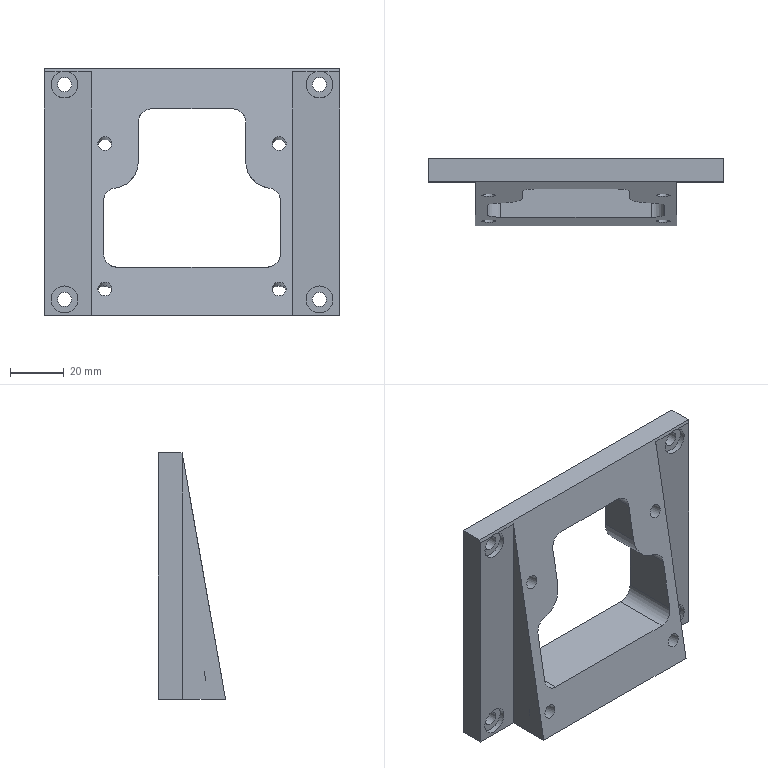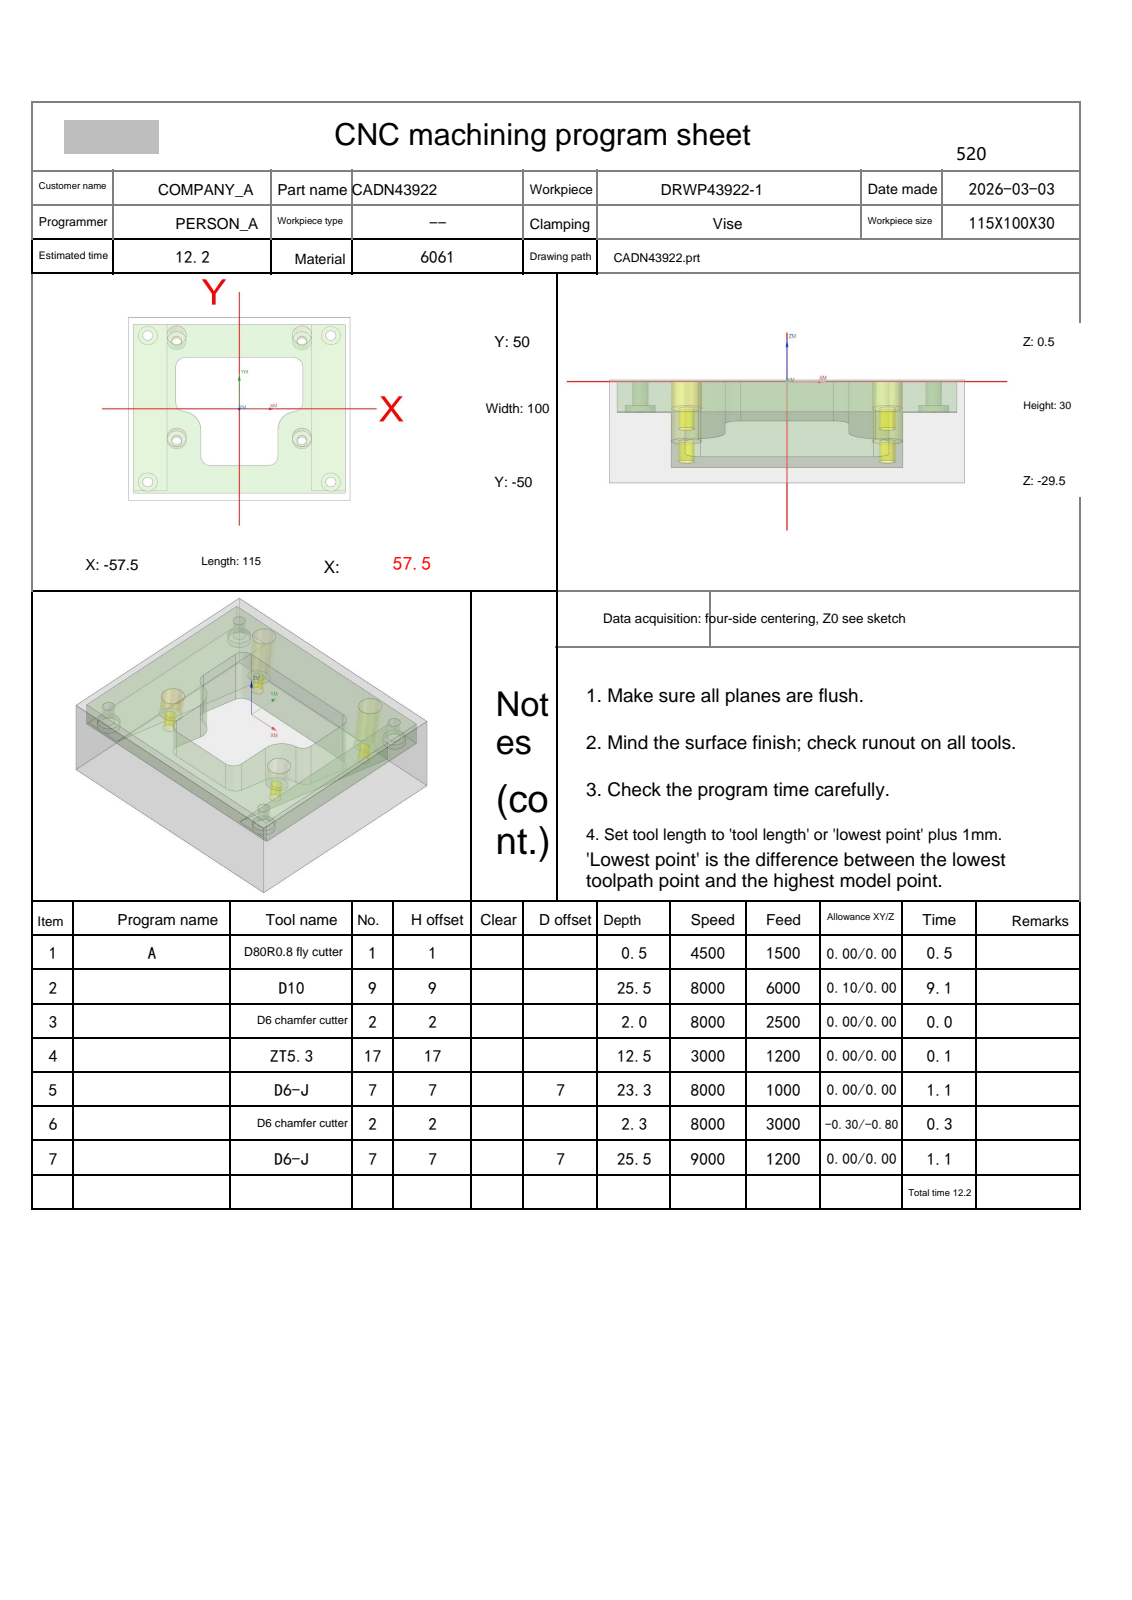NC program | NX | posted by the shop | part box 110 x 25 x 92 mm
Lines 36 to 1047 of 4607:
N2 T09 M06
(D10  D=10. R=0. H=09 ce=0.10 di=0.00)
G00 G90 G54 X0.0 Y-51.1 M03 S8000
G43 H09 Z50.
M08
Z.5
G01 X-55. Z.399 F6000.
G02 X-60.1 Y-46. Z.385 I0.0 J5.1
G01 Y46. Z.217
G02 X-55. Y51.1 Z.202 I5.1 J0.0
G01 X55. Z.001
G02 X60.1 Y46. Z-.014 I0.0 J-5.1
G01 Y-46. Z-.182
G02 X55. Y-51.1 Z-.196 I-5.1 J0.0
G01 X-55. Z-.397
G02 X-60.1 Y-46. Z-.412 I0.0 J5.1
G01 Y46. Z-.58
G02 X-55. Y51.1 Z-.595 I5.1 J0.0
G01 X55. Z-.796
G02 X60.1 Y46. Z-.81 I0.0 J-5.1
G01 Y-46. Z-.979
G02 X55. Y-51.1 Z-.993 I-5.1 J0.0
G01 X-55. Z-1.194
G02 X-60.1 Y-46. Z-1.209 I0.0 J5.1
G01 Y46. Z-1.377
G02 X-55. Y51.1 Z-1.392 I5.1 J0.0
G01 X55. Z-1.593
G02 X60.1 Y46. Z-1.607 I0.0 J-5.1
G01 Y-46. Z-1.775
G02 X55. Y-51.1 Z-1.79 I-5.1 J0.0
G01 X-55. Z-1.991
G02 X-60.1 Y-46. Z-2.006 I0.0 J5.1
G01 Y46. Z-2.174
G02 X-55. Y51.1 Z-2.189 I5.1 J0.0
G01 X55. Z-2.39
G02 X60.1 Y46. Z-2.404 I0.0 J-5.1
G01 Y-46. Z-2.572
G02 X55. Y-51.1 Z-2.587 I-5.1 J0.0
G01 X-55. Z-2.788
G02 X-60.1 Y-46. Z-2.803 I0.0 J5.1
G01 Y46. Z-2.971
G02 X-55. Y51.1 Z-2.985 I5.1 J0.0
G01 X55. Z-3.186
G02 X60.1 Y46. Z-3.201 I0.0 J-5.1
G01 Y-46. Z-3.369
G02 X55. Y-51.1 Z-3.384 I-5.1 J0.0
G01 X-55. Z-3.585
G02 X-60.1 Y-46. Z-3.6 I0.0 J5.1
G01 Y46. Z-3.768
G02 X-55. Y51.1 Z-3.782 I5.1 J0.0
G01 X55. Z-3.983
G02 X60.1 Y46. Z-3.998 I0.0 J-5.1
G01 Y-46. Z-4.166
G02 X55. Y-51.1 Z-4.181 I-5.1 J0.0
G01 X-55. Z-4.382
G02 X-60.1 Y-46. Z-4.396 I0.0 J5.1
G01 Y46. Z-4.565
G02 X-55. Y51.1 Z-4.579 I5.1 J0.0
G01 X55. Z-4.78
G02 X60.1 Y46. Z-4.795 I0.0 J-5.1
G01 Y-46. Z-4.963
G02 X55. Y-51.1 Z-4.978 I-5.1 J0.0
G01 X-55. Z-5.179
G02 X-60.1 Y-46. Z-5.193 I0.0 J5.1
G01 Y46. Z-5.361
G02 X-55. Y51.1 Z-5.376 I5.1 J0.0
G01 X55. Z-5.577
G02 X60.1 Y46. Z-5.592 I0.0 J-5.1
G01 Y-46. Z-5.76
G02 X55. Y-51.1 Z-5.774 I-5.1 J0.0
G01 X-55. Z-5.976
G02 X-60.1 Y-46. Z-5.99 I0.0 J5.1
G01 Y46. Z-6.158
G02 X-55. Y51.1 Z-6.173 I5.1 J0.0
G01 X55. Z-6.374
G02 X60.1 Y46. Z-6.389 I0.0 J-5.1
G01 Y-46. Z-6.557
G02 X55. Y-51.1 Z-6.571 I-5.1 J0.0
G01 X-55. Z-6.772
G02 X-60.1 Y-46. Z-6.787 I0.0 J5.1
G01 Y46. Z-6.955
G02 X-55. Y51.1 Z-6.97 I5.1 J0.0
G01 X55. Z-7.171
G02 X60.1 Y46. Z-7.185 I0.0 J-5.1
G01 Y-46. Z-7.354
G02 X55. Y-51.1 Z-7.368 I-5.1 J0.0
G01 X-55. Z-7.569
G02 X-60.1 Y-46. Z-7.584 I0.0 J5.1
G01 Y46. Z-7.752
G02 X-55. Y51.1 Z-7.767 I5.1 J0.0
G01 X55. Z-7.968
G02 X60.1 Y46. Z-7.982 I0.0 J-5.1
G01 Y-46. Z-8.15
G02 X55. Y-51.1 Z-8.165 I-5.1 J0.0
G01 X-55. Z-8.366
G02 X-60.1 Y-46. Z-8.381 I0.0 J5.1
G01 Y46. Z-8.549
G02 X-55. Y51.1 Z-8.564 I5.1 J0.0
G01 X55. Z-8.765
G02 X60.1 Y46. Z-8.779 I0.0 J-5.1
G01 Y-46. Z-8.947
G02 X55. Y-51.1 Z-8.962 I-5.1 J0.0
G01 X-55. Z-9.163
G02 X-60.1 Y-46. Z-9.178 I0.0 J5.1
G01 Y46. Z-9.346
G02 X-55. Y51.1 Z-9.36 I5.1 J0.0
G01 X55. Z-9.561
G02 X60.1 Y46. Z-9.576 I0.0 J-5.1
G01 Y-46. Z-9.744
G02 X55. Y-51.1 Z-9.759 I-5.1 J0.0
G01 X-55. Z-9.96
G02 X-60.1 Y-46. Z-9.975 I0.0 J5.1
G01 Y46. Z-10.143
G02 X-55. Y51.1 Z-10.157 I5.1 J0.0
G01 X55. Z-10.358
G02 X60.1 Y46. Z-10.373 I0.0 J-5.1
G01 Y-46. Z-10.541
G02 X55. Y-51.1 Z-10.556 I-5.1 J0.0
G01 X-55. Z-10.757
G02 X-60.1 Y-46. Z-10.771 I0.0 J5.1
G01 Y46. Z-10.94
G02 X-55. Y51.1 Z-10.954 I5.1 J0.0
G01 X55. Z-11.155
G02 X60.1 Y46. Z-11.17 I0.0 J-5.1
G01 Y-46. Z-11.338
G02 X55. Y-51.1 Z-11.353 I-5.1 J0.0
G01 X-55. Z-11.554
G02 X-60.1 Y-46. Z-11.568 I0.0 J5.1
G01 Y46. Z-11.736
G02 X-55. Y51.1 Z-11.751 I5.1 J0.0
G01 X55. Z-11.952
G02 X60.1 Y46. Z-11.967 I0.0 J-5.1
G01 Y-46. Z-12.135
G02 X55. Y-51.1 Z-12.149 I-5.1 J0.0
G01 X-55. Z-12.351
G02 X-60.1 Y-46. Z-12.365 I0.0 J5.1
G01 Y46. Z-12.533
G02 X-55. Y51.1 Z-12.548 I5.1 J0.0
G01 X55. Z-12.749
G02 X60.1 Y46. Z-12.764 I0.0 J-5.1
G01 Y-46. Z-12.932
G02 X55. Y-51.1 Z-12.946 I-5.1 J0.0
G01 X-55. Z-13.147
G02 X-60.1 Y-46. Z-13.162 I0.0 J5.1
G01 Y46. Z-13.33
G02 X-55. Y51.1 Z-13.345 I5.1 J0.0
G01 X55. Z-13.546
G02 X60.1 Y46. Z-13.56 I0.0 J-5.1
G01 Y-46. Z-13.729
G02 X55. Y-51.1 Z-13.743 I-5.1 J0.0
G01 X-55. Z-13.944
G02 X-60.1 Y-46. Z-13.959 I0.0 J5.1
G01 Y46. Z-14.127
G02 X-55. Y51.1 Z-14.142 I5.1 J0.0
G01 X55. Z-14.343
G02 X60.1 Y46. Z-14.357 I0.0 J-5.1
G01 Y-46. Z-14.525
G02 X55. Y-51.1 Z-14.54 I-5.1 J0.0
G01 X-55. Z-14.741
G02 X-60.1 Y-46. Z-14.756 I0.0 J5.1
G01 Y46. Z-14.924
G02 X-55. Y51.1 Z-14.939 I5.1 J0.0
G01 X55. Z-15.14
G02 X60.1 Y46. Z-15.154 I0.0 J-5.1
G01 Y-46. Z-15.322
G02 X55. Y-51.1 Z-15.337 I-5.1 J0.0
G01 X-55. Z-15.538
G02 X-60.1 Y-46. Z-15.553 I0.0 J5.1
G01 Y46. Z-15.721
G02 X-55. Y51.1 Z-15.735 I5.1 J0.0
G01 X55. Z-15.936
G02 X60.1 Y46. Z-15.951 I0.0 J-5.1
G01 Y-46. Z-16.119
G02 X55. Y-51.1 Z-16.134 I-5.1 J0.0
G01 X-55. Z-16.335
G02 X-60.1 Y-46. Z-16.35 I0.0 J5.1
G01 Y46. Z-16.518
G02 X-55. Y51.1 Z-16.532 I5.1 J0.0
G01 X55. Z-16.733
G02 X60.1 Y46. Z-16.748 I0.0 J-5.1
G01 Y-46. Z-16.916
G02 X55. Y-51.1 Z-16.931 I-5.1 J0.0
G01 X-55. Z-17.132
G02 X-60.1 Y-46. Z-17.146 I0.0 J5.1
G01 Y46. Z-17.315
G02 X-55. Y51.1 Z-17.329 I5.1 J0.0
G01 X55. Z-17.53
G02 X60.1 Y46. Z-17.545 I0.0 J-5.1
G01 Y-46. Z-17.713
G02 X55. Y-51.1 Z-17.728 I-5.1 J0.0
G01 X-55. Z-17.929
G02 X-60.1 Y-46. Z-17.943 I0.0 J5.1
G01 Y46. Z-18.111
G02 X-55. Y51.1 Z-18.126 I5.1 J0.0
G01 X55. Z-18.327
G02 X60.1 Y46. Z-18.342 I0.0 J-5.1
G01 Y-46. Z-18.51
G02 X55. Y-51.1 Z-18.524 I-5.1 J0.0
G01 X-55. Z-18.726
G02 X-60.1 Y-46. Z-18.74 I0.0 J5.1
G01 Y46. Z-18.908
G02 X-55. Y51.1 Z-18.923 I5.1 J0.0
G01 X55. Z-19.124
G02 X60.1 Y46. Z-19.139 I0.0 J-5.1
G01 Y-46. Z-19.307
G02 X55. Y-51.1 Z-19.321 I-5.1 J0.0
G01 X-55. Z-19.522
G02 X-60.1 Y-46. Z-19.537 I0.0 J5.1
G01 Y46. Z-19.705
G02 X-55. Y51.1 Z-19.72 I5.1 J0.0
G01 X55. Z-19.921
G02 X60.1 Y46. Z-19.935 I0.0 J-5.1
G01 Y-46. Z-20.104
G02 X55. Y-51.1 Z-20.118 I-5.1 J0.0
G01 X-55. Z-20.319
G02 X-60.1 Y-46. Z-20.334 I0.0 J5.1
G01 Y46. Z-20.502
G02 X-55. Y51.1 Z-20.517 I5.1 J0.0
G01 X55. Z-20.718
G02 X60.1 Y46. Z-20.732 I0.0 J-5.1
G01 Y-46. Z-20.9
G02 X55. Y-51.1 Z-20.915 I-5.1 J0.0
G01 X-55. Z-21.116
G02 X-60.1 Y-46. Z-21.131 I0.0 J5.1
G01 Y46. Z-21.299
G02 X-55. Y51.1 Z-21.314 I5.1 J0.0
G01 X55. Z-21.515
G02 X60.1 Y46. Z-21.529 I0.0 J-5.1
G01 Y-46. Z-21.697
G02 X55. Y-51.1 Z-21.712 I-5.1 J0.0
G01 X-55. Z-21.913
G02 X-60.1 Y-46. Z-21.928 I0.0 J5.1
G01 Y46. Z-22.096
G02 X-55. Y51.1 Z-22.11 I5.1 J0.0
G01 X55. Z-22.311
G02 X60.1 Y46. Z-22.326 I0.0 J-5.1
G01 Y-46. Z-22.494
G02 X55. Y-51.1 Z-22.509 I-5.1 J0.0
G01 X-55. Z-22.71
G02 X-60.1 Y-46. Z-22.725 I0.0 J5.1
G01 Y46. Z-22.893
G02 X-55. Y51.1 Z-22.907 I5.1 J0.0
G01 X55. Z-23.108
G02 X60.1 Y46. Z-23.123 I0.0 J-5.1
G01 Y-46. Z-23.291
G02 X55. Y-51.1 Z-23.306 I-5.1 J0.0
G01 X-55. Z-23.507
G02 X-60.1 Y-46. Z-23.521 I0.0 J5.1
G01 Y46. Z-23.69
G02 X-55. Y51.1 Z-23.704 I5.1 J0.0
G01 X55. Z-23.905
G02 X60.1 Y46. Z-23.92 I0.0 J-5.1
G01 Y-46. Z-24.088
G02 X55. Y-51.1 Z-24.103 I-5.1 J0.0
G01 X-55. Z-24.304
G02 X-60.1 Y-46. Z-24.318 I0.0 J5.1
G01 Y46. Z-24.486
G02 X-55. Y51.1 Z-24.501 I5.1 J0.0
G01 X55. Z-24.702
G02 X60.1 Y46. Z-24.717 I0.0 J-5.1
G01 Y-46. Z-24.885
G02 X55. Y-51.1 Z-24.899 I-5.1 J0.0
G01 X0.0 Z-25.
X-55.
G02 X-60.1 Y-46. I0.0 J5.1
G01 Y46.
G02 X-55. Y51.1 I5.1 J0.0
G01 X55.
G02 X60.1 Y46. I0.0 J-5.1
G01 Y-46.
G02 X55. Y-51.1 I-5.1 J0.0
G01 X0.0
X-.5
Z-24.
G00 Z50.
G00 G90 X-1.466 Y13.145 M03 S8000
Z10.5
Z1.5
G02 X-1.466 Y13.145 Z.018 I1.466 J4.255 F4000.
X-2.587 Y21.082 Z-.5 I1.466 J4.255
G01 X0.0 Y22.9
X27.9
Y3.587
G03 X14.9 Y-11.366 I2.1 J-14.953
G01 Y-25.9
X-14.9
Y-11.366
G03 X-27.9 Y3.587 I-15.1 J0.0
G01 Y22.9
X1.986
G02 X2.799 Y22.482 I0.0 J-1.
G01 X7.201 Y16.318
G03 X8.014 Y15.9 I.814 J.582
G01 X19.901
G02 X20.9 Y14.901 I-.001 J-1.
G01 Y13.66
G02 X20.631 Y12.978 I-1. J0.0
G01 X19.569 Y11.842
G03 X19.31 Y11.298 I.731 J-.683
G02 X17.61 Y9.268 I-2.476 J.347
G01 X10.909 Y7.08
G02 X10.133 Y6.957 I-.776 J2.377
X7.633 Y9.457 I0.0 J2.5
X9.357 Y11.833 I2.5 J0.0
G01 X16.058 Y14.021
G02 X16.834 Y14.145 I.776 J-2.377
X18.754 Y13.246 I0.0 J-2.5
G03 X18.916 Y13.091 I.768 J.64
G01 X20.507 Y11.876
G02 X20.9 Y11.082 I-.607 J-.795
G01 Y9.408
G02 X20.338 Y8.51 I-1. J.001
G03 X7.9 Y-11.366 I9.662 J-19.876
G01 Y-17.901
G02 X6.901 Y-18.9 I-1. J.001
G01 X-6.901
G02 X-7.9 Y-17.901 I.001 J1.
G01 Y-11.366
G03 X-20.338 Y8.51 I-22.1 J0.0
G02 X-20.9 Y9.408 I.438 J.899
G01 Y11.081
G02 X-20.507 Y11.876 I1. J0.0
G01 X-18.915 Y13.091
G03 X-18.754 Y13.245 I-.607 J.795
G02 X-16.834 Y14.145 I1.921 J-1.6
X-16.058 Y14.021 I0.0 J-2.5
G01 X-9.357 Y11.833
G02 X-7.633 Y9.457 I-.776 J-2.377
X-10.133 Y6.957 I-2.5 J0.0
X-10.909 Y7.08 I0.0 J2.5
G01 X-17.61 Y9.268
G02 X-19.31 Y11.298 I.776 J2.377
G03 X-19.569 Y11.842 I-.99 J-.139
G01 X-20.631 Y12.978
G02 X-20.9 Y13.66 I.731 J.682
G01 Y14.901
G02 X-19.901 Y15.9 I1. J-.001
G01 X1.975
G02 X2.798 Y15.468 I0.0 J-1.
G01 X7.38 Y8.827
G03 X7.538 Y8.648 I.823 J.568
G02 X7.874 Y7.9 I-.664 J-.748
X7.643 Y7.261 I-1. J0.0
G03 X.902 Y-11.012 I22.357 J-18.627
G02 X.002 Y-11.9 I-.9 J.012
G01 X-.004
G02 X-.902 Y-11.012 I.001 J.9
G03 X-7.643 Y7.261 I-29.098 J-.354
G02 X-7.874 Y7.9 I.769 J.639
X-6.875 Y8.9 I1. J0.0
G01 X5.
X5.5
G03 X12.5 Y15.9 I0.0 J7.
G01 Z.7
G00 Z3.
G01 X-1.466 Y13.145 F6000.
G00 Z1.
G02 X-1.466 Y13.145 Z-.482 I1.466 J4.255 F4000.
X-2.587 Y21.082 Z-1. I1.466 J4.255
G01 X0.0 Y22.9
X27.9
Y3.587
G03 X14.9 Y-11.366 I2.1 J-14.953
G01 Y-25.9
X-14.9
Y-11.366
G03 X-27.9 Y3.587 I-15.1 J0.0
G01 Y22.9
X5.
G02 X5.971 Y22.138 I0.0 J-1.
G01 X7.313 Y16.662
G03 X8.284 Y15.9 I.971 J.238
G01 X19.901
G02 X20.9 Y14.901 I-.001 J-1.
G01 Y13.66
G02 X20.631 Y12.978 I-1. J0.0
G01 X19.569 Y11.842
G03 X19.31 Y11.298 I.731 J-.683
G02 X17.61 Y9.268 I-2.476 J.347
G01 X10.909 Y7.08
G02 X10.133 Y6.957 I-.776 J2.377
X7.633 Y9.457 I0.0 J2.5
X9.357 Y11.833 I2.5 J0.0
G01 X16.058 Y14.021
G02 X16.834 Y14.145 I.776 J-2.377
X18.754 Y13.246 I0.0 J-2.5
G03 X18.916 Y13.091 I.768 J.64
G01 X20.507 Y11.876
G02 X20.9 Y11.082 I-.607 J-.795
G01 Y9.408
G02 X20.338 Y8.51 I-1. J.001
G03 X7.9 Y-11.366 I9.662 J-19.876
G01 Y-17.901
G02 X6.901 Y-18.9 I-1. J.001
G01 X-6.901
G02 X-7.9 Y-17.901 I.001 J1.
G01 Y-11.366
G03 X-20.338 Y8.51 I-22.1 J0.0
G02 X-20.9 Y9.408 I.438 J.899
G01 Y11.081
G02 X-20.507 Y11.876 I1. J0.0
G01 X-18.915 Y13.091
G03 X-18.754 Y13.245 I-.607 J.795
G02 X-16.834 Y14.145 I1.921 J-1.6
X-16.058 Y14.021 I0.0 J-2.5
G01 X-9.357 Y11.833
G02 X-7.633 Y9.457 I-.776 J-2.377
X-10.133 Y6.957 I-2.5 J0.0
X-10.909 Y7.08 I0.0 J2.5
G01 X-17.61 Y9.268
G02 X-19.31 Y11.298 I.776 J2.377
G03 X-19.569 Y11.842 I-.99 J-.139
G01 X-20.631 Y12.978
G02 X-20.9 Y13.66 I.731 J.682
G01 Y14.901
G02 X-19.901 Y15.9 I1. J-.001
G01 X1.975
G02 X2.798 Y15.468 I0.0 J-1.
G01 X7.38 Y8.827
G03 X7.538 Y8.648 I.823 J.568
G02 X7.874 Y7.9 I-.664 J-.748
X7.643 Y7.261 I-1. J0.0
G03 X.902 Y-11.012 I22.357 J-18.627
G02 X.002 Y-11.9 I-.9 J.012
G01 X-.003
G02 X-.902 Y-11.012 I.001 J.9
G03 X-7.643 Y7.261 I-29.098 J-.354
G02 X-7.874 Y7.9 I.769 J.639
X-6.875 Y8.9 I1. J0.0
G01 X5.
X5.5
G03 X12.5 Y15.9 I0.0 J7.
G01 Z.2
G00 Z2.5
G01 X-1.466 Y13.145 F6000.
G00 Z.5
G02 X-1.466 Y13.145 Z-.982 I1.466 J4.255 F4000.
X-2.587 Y21.082 Z-1.5 I1.466 J4.255
G01 X0.0 Y22.9
X27.9
Y3.587
G03 X14.9 Y-11.366 I2.1 J-14.953
G01 Y-25.9
X-14.9
Y-11.366
G03 X-27.9 Y3.587 I-15.1 J0.0
G01 Y22.9
X5.
G02 X5.971 Y22.138 I0.0 J-1.
G01 X7.313 Y16.662
G03 X8.284 Y15.9 I.971 J.238
G01 X19.901
G02 X20.9 Y14.901 I-.001 J-1.
G01 Y13.66
G02 X20.631 Y12.978 I-1. J0.0
G01 X19.569 Y11.842
G03 X19.31 Y11.298 I.731 J-.683
G02 X17.61 Y9.268 I-2.476 J.347
G01 X10.909 Y7.08
G02 X10.133 Y6.957 I-.776 J2.377
X7.633 Y9.457 I0.0 J2.5
X9.357 Y11.833 I2.5 J0.0
G01 X16.058 Y14.021
G02 X16.834 Y14.145 I.776 J-2.377
X18.754 Y13.246 I0.0 J-2.5
G03 X18.916 Y13.091 I.768 J.64
G01 X20.507 Y11.876
G02 X20.9 Y11.082 I-.607 J-.795
G01 Y9.408
G02 X20.338 Y8.51 I-1. J.001
G03 X7.9 Y-11.366 I9.662 J-19.876
G01 Y-17.901
G02 X6.901 Y-18.9 I-1. J.001
G01 X-6.901
G02 X-7.9 Y-17.901 I.001 J1.
G01 Y-11.366
G03 X-20.338 Y8.51 I-22.1 J0.0
G02 X-20.9 Y9.408 I.438 J.899
G01 Y11.081
G02 X-20.507 Y11.876 I1. J0.0
G01 X-18.915 Y13.091
G03 X-18.754 Y13.245 I-.607 J.795
G02 X-16.834 Y14.145 I1.921 J-1.6
X-16.058 Y14.021 I0.0 J-2.5
G01 X-9.357 Y11.833
G02 X-7.633 Y9.457 I-.776 J-2.377
X-10.133 Y6.957 I-2.5 J0.0
X-10.909 Y7.08 I0.0 J2.5
G01 X-17.61 Y9.268
G02 X-19.31 Y11.298 I.776 J2.377
G03 X-19.569 Y11.842 I-.99 J-.139
G01 X-20.631 Y12.978
G02 X-20.9 Y13.66 I.731 J.682
G01 Y14.901
G02 X-19.901 Y15.9 I1. J-.001
G01 X1.975
G02 X2.798 Y15.468 I0.0 J-1.
G01 X7.38 Y8.827
G03 X7.538 Y8.648 I.823 J.568
G02 X7.874 Y7.9 I-.664 J-.748
X7.643 Y7.261 I-1. J0.0
G03 X.902 Y-11.012 I22.357 J-18.627
G02 X.002 Y-11.9 I-.9 J.012
G01 X-.003
G02 X-.902 Y-11.012 I.001 J.9
G03 X-7.643 Y7.261 I-29.098 J-.354
G02 X-7.874 Y7.9 I.769 J.639
X-6.875 Y8.9 I1. J0.0
G01 X5.
X5.5
G03 X12.5 Y15.9 I0.0 J7.
G01 Z-.3
G00 Z2.
G01 X-1.466 Y13.145 F6000.
G00 Z0.0
G02 X-1.466 Y13.145 Z-1.482 I1.466 J4.255 F4000.
X-2.587 Y21.082 Z-2. I1.466 J4.255
G01 X0.0 Y22.9
X27.9
Y3.587
G03 X14.9 Y-11.366 I2.1 J-14.953
G01 Y-25.9
X-14.9
Y-11.366
G03 X-27.9 Y3.587 I-15.1 J0.0
G01 Y22.9
X5.
G02 X5.971 Y22.138 I0.0 J-1.
G01 X7.313 Y16.662
G03 X8.284 Y15.9 I.971 J.238
G01 X19.901
G02 X20.9 Y14.901 I-.001 J-1.
G01 Y13.66
G02 X20.631 Y12.978 I-1. J0.0
G01 X19.569 Y11.842
G03 X19.31 Y11.298 I.731 J-.683
G02 X17.61 Y9.268 I-2.476 J.347
G01 X10.909 Y7.08
G02 X10.133 Y6.957 I-.776 J2.377
X7.633 Y9.457 I0.0 J2.5
X9.357 Y11.833 I2.5 J0.0
G01 X16.058 Y14.021
G02 X16.834 Y14.145 I.776 J-2.377
X18.754 Y13.246 I0.0 J-2.5
G03 X18.916 Y13.091 I.768 J.64
G01 X20.507 Y11.876
G02 X20.9 Y11.082 I-.607 J-.795
G01 Y9.408
G02 X20.338 Y8.51 I-1. J.001
G03 X7.9 Y-11.366 I9.662 J-19.876
G01 Y-17.901
G02 X6.901 Y-18.9 I-1. J.001
G01 X-6.901
G02 X-7.9 Y-17.901 I.001 J1.
G01 Y-11.366
G03 X-20.338 Y8.51 I-22.1 J0.0
G02 X-20.9 Y9.408 I.438 J.899
G01 Y11.081
G02 X-20.507 Y11.876 I1. J0.0
G01 X-18.915 Y13.091
G03 X-18.754 Y13.245 I-.607 J.795
G02 X-16.834 Y14.145 I1.921 J-1.6
X-16.058 Y14.021 I0.0 J-2.5
G01 X-9.357 Y11.833
G02 X-7.633 Y9.457 I-.776 J-2.377
X-10.133 Y6.957 I-2.5 J0.0
X-10.909 Y7.08 I0.0 J2.5
G01 X-17.61 Y9.268
G02 X-19.31 Y11.298 I.776 J2.377
G03 X-19.569 Y11.842 I-.99 J-.139
G01 X-20.631 Y12.978
G02 X-20.9 Y13.66 I.731 J.682
G01 Y14.901
G02 X-19.901 Y15.9 I1. J-.001
G01 X1.975
G02 X2.798 Y15.468 I0.0 J-1.
G01 X7.38 Y8.827
G03 X7.538 Y8.648 I.823 J.568
G02 X7.874 Y7.9 I-.664 J-.748
X7.643 Y7.261 I-1. J0.0
G03 X.902 Y-11.012 I22.357 J-18.627
G02 X.002 Y-11.9 I-.9 J.012
G01 X-.003
G02 X-.902 Y-11.012 I.001 J.9
G03 X-7.643 Y7.261 I-29.098 J-.354
G02 X-7.874 Y7.9 I.769 J.639
X-6.875 Y8.9 I1. J0.0
G01 X5.
X5.5
G03 X12.5 Y15.9 I0.0 J7.
G01 Z-.8
G00 Z1.5
G01 X-1.466 Y13.145 F6000.
G00 Z-.5
G02 X-1.466 Y13.145 Z-1.982 I1.466 J4.255 F4000.
X-2.587 Y21.082 Z-2.5 I1.466 J4.255
G01 X0.0 Y22.9
X27.9
Y3.587
G03 X14.9 Y-11.366 I2.1 J-14.953
G01 Y-25.9
X-14.9
Y-11.366
G03 X-27.9 Y3.587 I-15.1 J0.0
G01 Y22.9
X5.
G02 X5.971 Y22.138 I0.0 J-1.
G01 X7.313 Y16.662
G03 X8.284 Y15.9 I.971 J.238
G01 X19.901
G02 X20.9 Y14.901 I-.001 J-1.
G01 Y13.66
G02 X20.631 Y12.978 I-1. J0.0
G01 X19.569 Y11.842
G03 X19.31 Y11.298 I.731 J-.683
G02 X17.61 Y9.268 I-2.476 J.347
G01 X10.909 Y7.08
G02 X10.133 Y6.957 I-.776 J2.377
X7.633 Y9.457 I0.0 J2.5
X9.357 Y11.833 I2.5 J0.0
G01 X16.058 Y14.021
G02 X16.834 Y14.145 I.776 J-2.377
X18.754 Y13.246 I0.0 J-2.5
G03 X18.916 Y13.091 I.768 J.64
G01 X20.507 Y11.876
G02 X20.9 Y11.082 I-.607 J-.795
G01 Y9.408
G02 X20.338 Y8.51 I-1. J.001
G03 X7.9 Y-11.366 I9.662 J-19.876
G01 Y-17.901
G02 X6.901 Y-18.9 I-1. J.001
G01 X-6.901
G02 X-7.9 Y-17.901 I.001 J1.
G01 Y-11.366
G03 X-20.338 Y8.51 I-22.1 J0.0
G02 X-20.9 Y9.408 I.438 J.899
G01 Y11.081
G02 X-20.507 Y11.876 I1. J0.0
G01 X-18.915 Y13.091
G03 X-18.754 Y13.245 I-.607 J.795
G02 X-16.834 Y14.145 I1.921 J-1.6
X-16.058 Y14.021 I0.0 J-2.5
G01 X-9.357 Y11.833
G02 X-7.633 Y9.457 I-.776 J-2.377
X-10.133 Y6.957 I-2.5 J0.0
X-10.909 Y7.08 I0.0 J2.5
G01 X-17.61 Y9.268
G02 X-19.31 Y11.298 I.776 J2.377
G03 X-19.569 Y11.842 I-.99 J-.139
G01 X-20.631 Y12.978
G02 X-20.9 Y13.66 I.731 J.682
G01 Y14.901
G02 X-19.901 Y15.9 I1. J-.001
G01 X1.975
G02 X2.798 Y15.468 I0.0 J-1.
G01 X7.38 Y8.827
G03 X7.538 Y8.648 I.823 J.568
G02 X7.874 Y7.9 I-.664 J-.748
X7.643 Y7.261 I-1. J0.0
G03 X.902 Y-11.012 I22.357 J-18.627
G02 X.002 Y-11.9 I-.9 J.012
G01 X-.003
G02 X-.902 Y-11.012 I.001 J.9
G03 X-7.643 Y7.261 I-29.098 J-.354
G02 X-7.874 Y7.9 I.769 J.639
X-6.875 Y8.9 I1. J0.0
G01 X5.
X5.5
G03 X12.5 Y15.9 I0.0 J7.
G01 Z-1.3
G00 Z1.
G01 X-1.466 Y13.145 F6000.
G00 Z-1.
G02 X-1.466 Y13.145 Z-2.482 I1.466 J4.255 F4000.
X-2.587 Y21.082 Z-3. I1.466 J4.255
G01 X0.0 Y22.9
X27.9
Y3.587
G03 X14.9 Y-11.366 I2.1 J-14.953
G01 Y-25.9
X-14.9
Y-11.366
G03 X-27.9 Y3.587 I-15.1 J0.0
G01 Y22.9
X5.
G02 X5.971 Y22.138 I0.0 J-1.
G01 X7.313 Y16.662
G03 X8.284 Y15.9 I.971 J.238
G01 X19.901
G02 X20.9 Y14.901 I-.001 J-1.
G01 Y13.66
G02 X20.631 Y12.978 I-1. J0.0
G01 X19.569 Y11.842
G03 X19.31 Y11.298 I.731 J-.683
G02 X17.61 Y9.268 I-2.476 J.347
G01 X10.909 Y7.08
G02 X10.133 Y6.957 I-.776 J2.377
X7.633 Y9.457 I0.0 J2.5
X9.357 Y11.833 I2.5 J0.0
G01 X16.058 Y14.021
G02 X16.834 Y14.145 I.776 J-2.377
X18.754 Y13.246 I0.0 J-2.5
G03 X18.916 Y13.091 I.768 J.64
G01 X20.507 Y11.876
G02 X20.9 Y11.082 I-.607 J-.795
G01 Y9.408
G02 X20.338 Y8.51 I-1. J.001
G03 X7.9 Y-11.366 I9.662 J-19.876
G01 Y-17.901
G02 X6.901 Y-18.9 I-1. J.001
G01 X-6.901
G02 X-7.9 Y-17.901 I.001 J1.
G01 Y-11.366
G03 X-20.338 Y8.51 I-22.1 J0.0
G02 X-20.9 Y9.408 I.438 J.899
G01 Y11.081
G02 X-20.507 Y11.876 I1. J0.0
G01 X-18.915 Y13.091
G03 X-18.754 Y13.245 I-.607 J.795
G02 X-16.834 Y14.145 I1.921 J-1.6
X-16.058 Y14.021 I0.0 J-2.5
G01 X-9.357 Y11.833
G02 X-7.633 Y9.457 I-.776 J-2.377
X-10.133 Y6.957 I-2.5 J0.0
X-10.909 Y7.08 I0.0 J2.5
G01 X-17.61 Y9.268
G02 X-19.31 Y11.298 I.776 J2.377
G03 X-19.569 Y11.842 I-.99 J-.139
G01 X-20.631 Y12.978
G02 X-20.9 Y13.66 I.731 J.682
G01 Y14.901
G02 X-19.901 Y15.9 I1. J-.001
G01 X1.975
G02 X2.798 Y15.468 I0.0 J-1.
G01 X7.38 Y8.827
G03 X7.538 Y8.648 I.823 J.568
G02 X7.874 Y7.9 I-.664 J-.748
X7.643 Y7.261 I-1. J0.0
G03 X.902 Y-11.012 I22.357 J-18.627
G02 X.002 Y-11.9 I-.9 J.012
G01 X-.003
G02 X-.902 Y-11.012 I.001 J.9
G03 X-7.643 Y7.261 I-29.098 J-.354
G02 X-7.874 Y7.9 I.769 J.639
X-6.875 Y8.9 I1. J0.0
G01 X5.
X5.5
G03 X12.5 Y15.9 I0.0 J7.
G01 Z-1.8
G00 Z.5
G01 X-1.466 Y13.145 F6000.
G00 Z-1.5
G02 X-1.466 Y13.145 Z-2.982 I1.466 J4.255 F4000.
X-2.587 Y21.082 Z-3.5 I1.466 J4.255
G01 X0.0 Y22.9
X27.9
Y3.587
G03 X14.9 Y-11.366 I2.1 J-14.953
G01 Y-25.9
X-14.9
Y-11.366
G03 X-27.9 Y3.587 I-15.1 J0.0
G01 Y22.9
X5.
G02 X5.971 Y22.138 I0.0 J-1.
G01 X7.313 Y16.662
G03 X8.284 Y15.9 I.971 J.238
G01 X19.901
G02 X20.9 Y14.901 I-.001 J-1.
G01 Y13.66
G02 X20.631 Y12.978 I-1. J0.0
G01 X19.569 Y11.842
G03 X19.31 Y11.298 I.731 J-.683
G02 X17.61 Y9.268 I-2.476 J.347
G01 X10.909 Y7.08
G02 X10.133 Y6.957 I-.776 J2.377
X7.633 Y9.457 I0.0 J2.5
X9.357 Y11.833 I2.5 J0.0
G01 X16.058 Y14.021
G02 X16.834 Y14.145 I.776 J-2.377
X18.754 Y13.246 I0.0 J-2.5
G03 X18.916 Y13.091 I.768 J.64
G01 X20.507 Y11.876
G02 X20.9 Y11.082 I-.607 J-.795
G01 Y9.408
G02 X20.338 Y8.51 I-1. J.001
G03 X7.9 Y-11.366 I9.662 J-19.876
G01 Y-17.901
G02 X6.901 Y-18.9 I-1. J.001
G01 X-6.901
G02 X-7.9 Y-17.901 I.001 J1.
G01 Y-11.366
G03 X-20.338 Y8.51 I-22.1 J0.0
G02 X-20.9 Y9.408 I.438 J.899
G01 Y11.081
G02 X-20.507 Y11.876 I1. J0.0
G01 X-18.915 Y13.091
G03 X-18.754 Y13.245 I-.607 J.795
G02 X-16.834 Y14.145 I1.921 J-1.6
X-16.058 Y14.021 I0.0 J-2.5
G01 X-9.357 Y11.833
G02 X-7.633 Y9.457 I-.776 J-2.377
X-10.133 Y6.957 I-2.5 J0.0
X-10.909 Y7.08 I0.0 J2.5
G01 X-17.61 Y9.268
G02 X-19.31 Y11.298 I.776 J2.377
G03 X-19.569 Y11.842 I-.99 J-.139
G01 X-20.631 Y12.978
G02 X-20.9 Y13.66 I.731 J.682
G01 Y14.901
G02 X-19.901 Y15.9 I1. J-.001
G01 X1.975
G02 X2.798 Y15.468 I0.0 J-1.
G01 X7.38 Y8.827
G03 X7.538 Y8.648 I.823 J.568
G02 X7.874 Y7.9 I-.664 J-.748
X7.643 Y7.261 I-1. J0.0
G03 X.902 Y-11.012 I22.357 J-18.627
G02 X.002 Y-11.9 I-.9 J.012
G01 X-.003
G02 X-.902 Y-11.012 I.001 J.9
G03 X-7.643 Y7.261 I-29.098 J-.354
G02 X-7.874 Y7.9 I.769 J.639
X-6.875 Y8.9 I1. J0.0
G01 X5.
X5.5
G03 X12.5 Y15.9 I0.0 J7.
G01 Z-2.3
G00 Z0.0
G01 X-1.466 Y13.145 F6000.
G00 Z-2.
G02 X-1.466 Y13.145 Z-3.482 I1.466 J4.255 F4000.
X-2.587 Y21.082 Z-4. I1.466 J4.255
G01 X0.0 Y22.9
X27.9
Y3.587
G03 X14.9 Y-11.366 I2.1 J-14.953
G01 Y-25.9
X-14.9
Y-11.366
G03 X-27.9 Y3.587 I-15.1 J0.0
G01 Y22.9
X5.
G02 X5.971 Y22.138 I0.0 J-1.
G01 X7.313 Y16.662
G03 X8.284 Y15.9 I.971 J.238
G01 X19.901
G02 X20.9 Y14.901 I-.001 J-1.
G01 Y13.66
G02 X20.631 Y12.978 I-1. J0.0
G01 X19.569 Y11.842
G03 X19.31 Y11.298 I.731 J-.683
G02 X17.61 Y9.268 I-2.476 J.347
G01 X10.909 Y7.08
G02 X10.133 Y6.957 I-.776 J2.377
X7.633 Y9.457 I0.0 J2.5
X9.357 Y11.833 I2.5 J0.0
G01 X16.058 Y14.021
G02 X16.834 Y14.145 I.776 J-2.377
X18.754 Y13.246 I0.0 J-2.5
G03 X18.916 Y13.091 I.768 J.64
G01 X20.507 Y11.876
G02 X20.9 Y11.082 I-.607 J-.795
G01 Y9.408
G02 X20.338 Y8.51 I-1. J.001
G03 X7.9 Y-11.366 I9.662 J-19.876
G01 Y-17.901
G02 X6.901 Y-18.9 I-1. J.001
G01 X-6.901
G02 X-7.9 Y-17.901 I.001 J1.
G01 Y-11.366
G03 X-20.338 Y8.51 I-22.1 J0.0
G02 X-20.9 Y9.408 I.438 J.899
G01 Y11.081
G02 X-20.507 Y11.876 I1. J0.0
G01 X-18.915 Y13.091
G03 X-18.754 Y13.245 I-.607 J.795
G02 X-16.834 Y14.145 I1.921 J-1.6
X-16.058 Y14.021 I0.0 J-2.5
G01 X-9.357 Y11.833
G02 X-7.633 Y9.457 I-.776 J-2.377
X-10.133 Y6.957 I-2.5 J0.0
X-10.909 Y7.08 I0.0 J2.5
G01 X-17.61 Y9.268
G02 X-19.31 Y11.298 I.776 J2.377
G03 X-19.569 Y11.842 I-.99 J-.139
G01 X-20.631 Y12.978
G02 X-20.9 Y13.66 I.731 J.682
G01 Y14.901
G02 X-19.901 Y15.9 I1. J-.001
G01 X1.975
G02 X2.798 Y15.468 I0.0 J-1.
G01 X7.38 Y8.827
G03 X7.538 Y8.648 I.823 J.568
G02 X7.874 Y7.9 I-.664 J-.748
X7.643 Y7.261 I-1. J0.0
G03 X.902 Y-11.012 I22.357 J-18.627
G02 X.002 Y-11.9 I-.9 J.012
G01 X-.003
G02 X-.902 Y-11.012 I.001 J.9
G03 X-7.643 Y7.261 I-29.098 J-.354
G02 X-7.874 Y7.9 I.769 J.639
X-6.875 Y8.9 I1. J0.0
G01 X5.
X5.5
G03 X12.5 Y15.9 I0.0 J7.
G01 Z-2.8
G00 Z-.5
G01 X-1.466 Y13.145 F6000.
G00 Z-2.5
G02 X-1.466 Y13.145 Z-3.982 I1.466 J4.255 F4000.
X-2.587 Y21.082 Z-4.5 I1.466 J4.255
G01 X0.0 Y22.9
X27.9
Y3.587
G03 X14.9 Y-11.366 I2.1 J-14.953
G01 Y-25.9
X-14.9
Y-11.366
G03 X-27.9 Y3.587 I-15.1 J0.0
G01 Y22.9
X5.
G02 X5.971 Y22.138 I0.0 J-1.
G01 X7.313 Y16.662
G03 X8.284 Y15.9 I.971 J.238
G01 X19.901
G02 X20.9 Y14.901 I-.001 J-1.
G01 Y13.66
G02 X20.631 Y12.978 I-1. J0.0
G01 X19.569 Y11.842
G03 X19.31 Y11.298 I.731 J-.683
G02 X17.61 Y9.268 I-2.476 J.347
G01 X10.909 Y7.08
G02 X10.133 Y6.957 I-.776 J2.377
X7.633 Y9.457 I0.0 J2.5
X9.357 Y11.833 I2.5 J0.0
G01 X16.058 Y14.021
G02 X16.834 Y14.145 I.776 J-2.377
X18.754 Y13.246 I0.0 J-2.5
G03 X18.916 Y13.091 I.768 J.64
G01 X20.507 Y11.876
G02 X20.9 Y11.082 I-.607 J-.795
G01 Y9.408
G02 X20.338 Y8.51 I-1. J.001
G03 X7.9 Y-11.366 I9.662 J-19.876
G01 Y-17.901
G02 X6.901 Y-18.9 I-1. J.001
G01 X-6.901
G02 X-7.9 Y-17.901 I.001 J1.
G01 Y-11.366
G03 X-20.338 Y8.51 I-22.1 J0.0
G02 X-20.9 Y9.408 I.438 J.899
G01 Y11.081
G02 X-20.507 Y11.876 I1. J0.0
G01 X-18.915 Y13.091
G03 X-18.754 Y13.245 I-.607 J.795
G02 X-16.834 Y14.145 I1.921 J-1.6
X-16.058 Y14.021 I0.0 J-2.5
G01 X-9.357 Y11.833
G02 X-7.633 Y9.457 I-.776 J-2.377
X-10.133 Y6.957 I-2.5 J0.0
X-10.909 Y7.08 I0.0 J2.5
G01 X-17.61 Y9.268
G02 X-19.31 Y11.298 I.776 J2.377
G03 X-19.569 Y11.842 I-.99 J-.139
G01 X-20.631 Y12.978
G02 X-20.9 Y13.66 I.731 J.682
G01 Y14.901
G02 X-19.901 Y15.9 I1. J-.001
G01 X1.975
G02 X2.798 Y15.468 I0.0 J-1.
G01 X7.38 Y8.827
G03 X7.538 Y8.648 I.823 J.568
G02 X7.874 Y7.9 I-.664 J-.748
X7.643 Y7.261 I-1. J0.0
G03 X.902 Y-11.012 I22.357 J-18.627
G02 X.002 Y-11.9 I-.9 J.012
G01 X-.003
G02 X-.902 Y-11.012 I.001 J.9
G03 X-7.643 Y7.261 I-29.098 J-.354
G02 X-7.874 Y7.9 I.769 J.639
X-6.875 Y8.9 I1. J0.0
G01 X5.
X5.5
G03 X12.5 Y15.9 I0.0 J7.
G01 Z-3.3
G00 Z-1.
G01 X-1.466 Y13.145 F6000.
G00 Z-3.
G02 X-1.466 Y13.145 Z-4.482 I1.466 J4.255 F4000.
X-2.587 Y21.082 Z-5. I1.466 J4.255
G01 X0.0 Y22.9
X27.9
Y3.587
G03 X14.9 Y-11.366 I2.1 J-14.953
G01 Y-25.9
X-14.9
Y-11.366
G03 X-27.9 Y3.587 I-15.1 J0.0
G01 Y22.9
X5.
G02 X5.971 Y22.138 I0.0 J-1.
G01 X7.313 Y16.662
G03 X8.284 Y15.9 I.971 J.238
G01 X19.901
G02 X20.9 Y14.901 I-.001 J-1.
G01 Y13.66
G02 X20.631 Y12.978 I-1. J0.0
G01 X19.569 Y11.842
G03 X19.31 Y11.298 I.731 J-.683
G02 X17.61 Y9.268 I-2.476 J.347
G01 X10.909 Y7.08